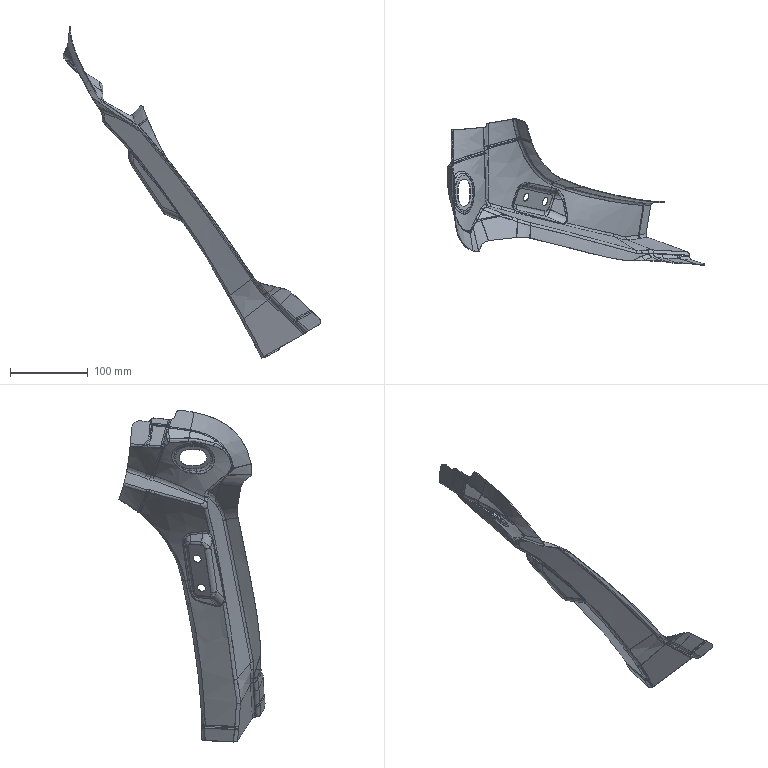Part | STEP file | FNA5401155 | 1 solid | 480 faces | box 332 x 187.997 x 427.512 mm | volume 56977 mm3 | spline 427 | sphere 24 | cylinder 21 | plane 8 | commonest cylinder face diameters 11 x4 20 x4 21.6 x4 12 x2 13.6 x2 600 x1